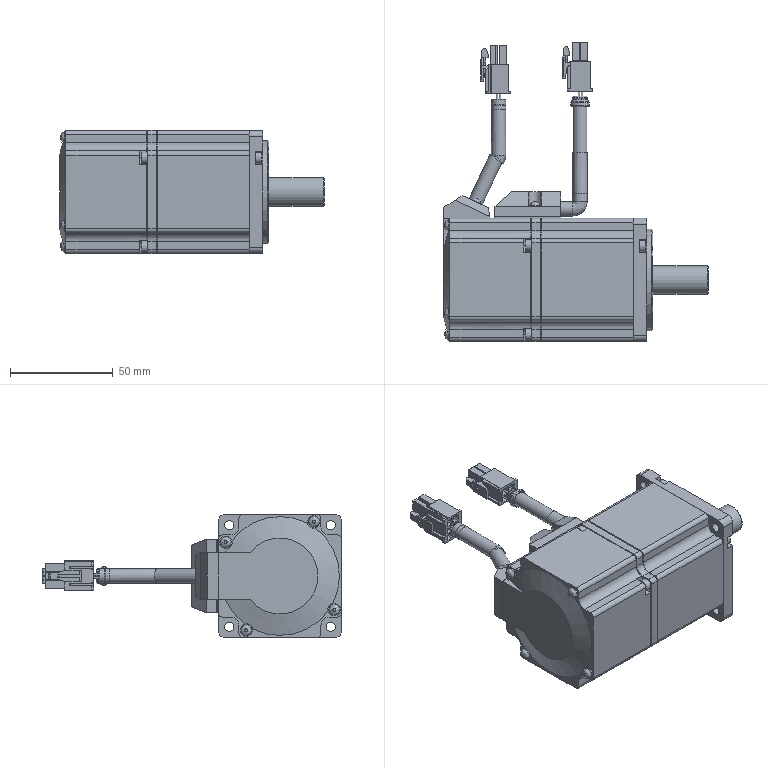Part | NX | 7 solids | 685 faces | box 129 x 145.8 x 60 mm | volume 349775 mm3 | plane 487 | cylinder 171 | spline 14 | cone 13 | commonest cylinder face diameters 4 x46 8 x24 0.6 x18 6.5 x12 1 x10 2.6 x10